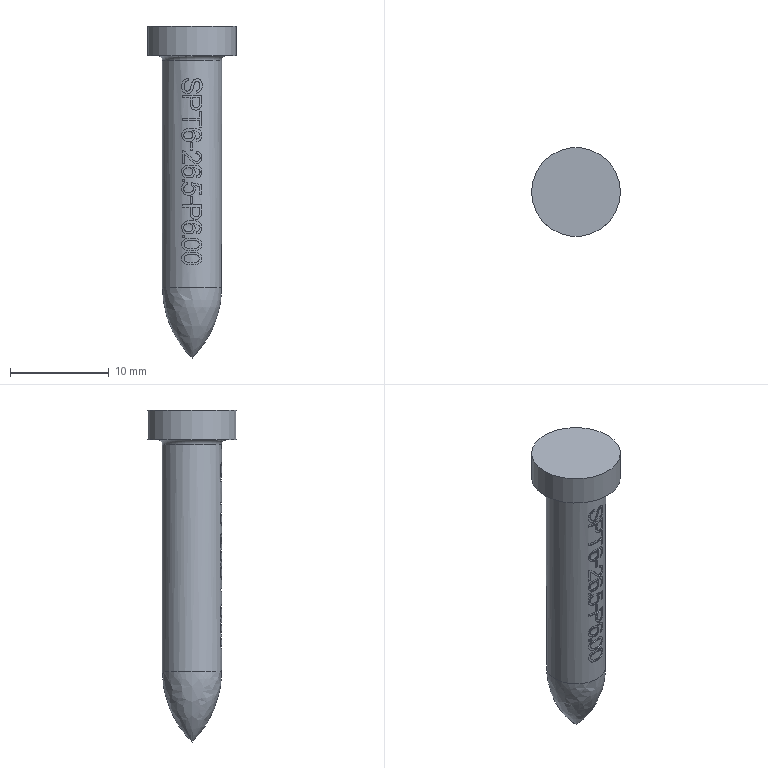Part | STEP file | PN_0062_id766_x_t | 1 solid | 196 faces | box 9 x 9 x 33.641 mm | volume 968.209 mm3 | plane 103 | cylinder 91 | torus 1 | spline 1 | commonest cylinder face diameters 5.8 x15 6 x8 0.688 x3 0.77 x3 0.792 x3 0.998 x3